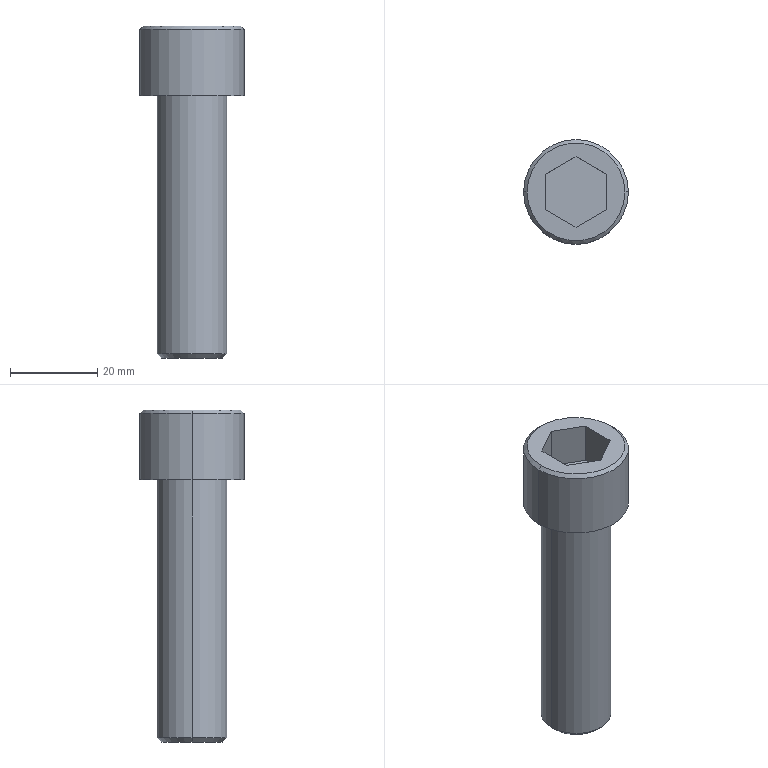Part | Creo | 1 solid | 18 faces | box 24 x 24 x 76 mm | volume 17625 mm3 | plane 10 | cylinder 4 | cone 4 | commonest cylinder face diameters 16 x2 24 x2
STEP:
#1=CARTESIAN_POINT('',(174.,251.,132.5));
#2=VERTEX_POINT('',#1);
#3=CARTESIAN_POINT('',(150.,251.,132.5));
#4=VERTEX_POINT('',#3);
#5=CARTESIAN_POINT('',(162.,251.,132.5));
#6=DIRECTION('',(0.,0.,-1.));
#7=DIRECTION('',(1.,0.,0.));
#8=AXIS2_PLACEMENT_3D('',#5,#6,#7);
#9=CIRCLE('',#8,12.);
#10=EDGE_CURVE('',#2,#4,#9,.T.);
#11=ORIENTED_EDGE('',*,*,#10,.F.);
#12=CARTESIAN_POINT('',(162.,251.,132.5));
#13=DIRECTION('',(0.,0.,-1.));
#14=DIRECTION('',(-1.,0.,0.));
#15=AXIS2_PLACEMENT_3D('',#12,#13,#14);
#16=CIRCLE('',#15,12.);
#17=EDGE_CURVE('',#4,#2,#16,.T.);
#18=ORIENTED_EDGE('',*,*,#17,.F.);
#19=EDGE_LOOP('',(#11,#18));
#20=FACE_OUTER_BOUND('',#19,.F.);
#21=CARTESIAN_POINT('',(154.,251.,132.5));
#22=VERTEX_POINT('',#21);
#23=CARTESIAN_POINT('',(170.,251.,132.5));
#24=VERTEX_POINT('',#23);
#25=CARTESIAN_POINT('',(162.,251.,132.5));
#26=DIRECTION('',(0.,0.,1.));
#27=DIRECTION('',(-1.,0.,0.));
#28=AXIS2_PLACEMENT_3D('',#25,#26,#27);
#29=CIRCLE('',#28,8.);
#30=EDGE_CURVE('',#22,#24,#29,.T.);
#31=ORIENTED_EDGE('',*,*,#30,.F.);
#32=CARTESIAN_POINT('',(162.,251.,132.5));
#33=DIRECTION('',(0.,0.,1.));
#34=DIRECTION('',(1.,0.,0.));
#35=AXIS2_PLACEMENT_3D('',#32,#33,#34);
#36=CIRCLE('',#35,8.);
#37=EDGE_CURVE('',#24,#22,#36,.T.);
#38=ORIENTED_EDGE('',*,*,#37,.F.);
#39=EDGE_LOOP('',(#31,#38));
#40=FACE_BOUND('',#39,.F.);
#41=CARTESIAN_POINT('',(162.,251.,132.5));
#42=DIRECTION('',(0.,0.,-1.));
#43=DIRECTION('',(-1.,0.,0.));
#44=AXIS2_PLACEMENT_3D('',#41,#42,#43);
#45=PLANE('',#44);
#46=ADVANCED_FACE('',(#20,#40),#45,.T.);
#47=CARTESIAN_POINT('',(170.,251.,73.5));
#48=VERTEX_POINT('',#47);
#49=CARTESIAN_POINT('',(154.,251.,73.5));
#50=VERTEX_POINT('',#49);
#51=CARTESIAN_POINT('',(162.,251.,73.5));
#52=DIRECTION('',(0.,0.,-1.));
#53=DIRECTION('',(1.,0.,0.));
#54=AXIS2_PLACEMENT_3D('',#51,#52,#53);
#55=CIRCLE('',#54,8.);
#56=EDGE_CURVE('',#48,#50,#55,.T.);
#57=ORIENTED_EDGE('',*,*,#56,.T.);
#58=CARTESIAN_POINT('',(154.,251.,132.5));
#59=DIRECTION('',(0.,0.,-1.));
#60=VECTOR('',#59,59.);
#61=LINE('',#58,#60);
#62=EDGE_CURVE('',#22,#50,#61,.T.);
#63=ORIENTED_EDGE('',*,*,#62,.F.);
#64=ORIENTED_EDGE('',*,*,#30,.T.);
#65=CARTESIAN_POINT('',(170.,251.,132.5));
#66=DIRECTION('',(0.,0.,-1.));
#67=VECTOR('',#66,59.);
#68=LINE('',#65,#67);
#69=EDGE_CURVE('',#24,#48,#68,.T.);
#70=ORIENTED_EDGE('',*,*,#69,.T.);
#71=EDGE_LOOP('',(#57,#63,#64,#70));
#72=FACE_OUTER_BOUND('',#71,.F.);
#73=CARTESIAN_POINT('',(162.,251.,150.5));
#74=DIRECTION('',(0.,0.,-1.));
#75=DIRECTION('',(-1.,0.,0.));
#76=AXIS2_PLACEMENT_3D('',#73,#74,#75);
#77=CYLINDRICAL_SURFACE('',#76,8.);
#78=ADVANCED_FACE('',(#72),#77,.T.);
#79=CARTESIAN_POINT('',(169.,251.,72.5));
#80=VERTEX_POINT('',#79);
#81=CARTESIAN_POINT('',(155.,251.,72.5));
#82=VERTEX_POINT('',#81);
#83=CARTESIAN_POINT('',(162.,251.,72.5));
#84=DIRECTION('',(0.,0.,-1.));
#85=DIRECTION('',(1.,0.,0.));
#86=AXIS2_PLACEMENT_3D('',#83,#84,#85);
#87=CIRCLE('',#86,7.);
#88=EDGE_CURVE('',#80,#82,#87,.T.);
#89=ORIENTED_EDGE('',*,*,#88,.T.);
#90=CARTESIAN_POINT('',(155.,251.,72.5));
#91=DIRECTION('',(-0.7071,0.,0.7071));
#92=VECTOR('',#91,1.414);
#93=LINE('',#90,#92);
#94=EDGE_CURVE('',#82,#50,#93,.T.);
#95=ORIENTED_EDGE('',*,*,#94,.T.);
#96=ORIENTED_EDGE('',*,*,#56,.F.);
#97=CARTESIAN_POINT('',(169.,251.,72.5));
#98=DIRECTION('',(0.7071,0.,0.7071));
#99=VECTOR('',#98,1.414);
#100=LINE('',#97,#99);
#101=EDGE_CURVE('',#80,#48,#100,.T.);
#102=ORIENTED_EDGE('',*,*,#101,.F.);
#103=EDGE_LOOP('',(#89,#95,#96,#102));
#104=FACE_OUTER_BOUND('',#103,.F.);
#105=CARTESIAN_POINT('',(162.,251.,73.));
#106=DIRECTION('',(0.,0.,1.));
#107=DIRECTION('',(1.,0.,0.));
#108=AXIS2_PLACEMENT_3D('',#105,#106,#107);
#109=CONICAL_SURFACE('',#108,7.5,45.);
#110=ADVANCED_FACE('',(#104),#109,.T.);
#111=CARTESIAN_POINT('',(162.,251.,72.5));
#112=DIRECTION('',(0.,0.,-1.));
#113=DIRECTION('',(-1.,0.,0.));
#114=AXIS2_PLACEMENT_3D('',#111,#112,#113);
#115=CIRCLE('',#114,7.);
#116=EDGE_CURVE('',#82,#80,#115,.T.);
#117=ORIENTED_EDGE('',*,*,#116,.F.);
#118=ORIENTED_EDGE('',*,*,#88,.F.);
#119=EDGE_LOOP('',(#117,#118));
#120=FACE_OUTER_BOUND('',#119,.F.);
#121=CARTESIAN_POINT('',(162.,251.,72.5));
#122=DIRECTION('',(0.,0.,-1.));
#123=DIRECTION('',(-1.,0.,0.));
#124=AXIS2_PLACEMENT_3D('',#121,#122,#123);
#125=PLANE('',#124);
#126=ADVANCED_FACE('',(#120),#125,.T.);
#127=ORIENTED_EDGE('',*,*,#116,.T.);
#128=ORIENTED_EDGE('',*,*,#101,.T.);
#129=CARTESIAN_POINT('',(162.,251.,73.5));
#130=DIRECTION('',(0.,0.,-1.));
#131=DIRECTION('',(-1.,0.,0.));
#132=AXIS2_PLACEMENT_3D('',#129,#130,#131);
#133=CIRCLE('',#132,8.);
#134=EDGE_CURVE('',#50,#48,#133,.T.);
#135=ORIENTED_EDGE('',*,*,#134,.F.);
#136=ORIENTED_EDGE('',*,*,#94,.F.);
#137=EDGE_LOOP('',(#127,#128,#135,#136));
#138=FACE_OUTER_BOUND('',#137,.F.);
#139=CARTESIAN_POINT('',(162.,251.,73.));
#140=DIRECTION('',(0.,0.,1.));
#141=DIRECTION('',(1.,0.,0.));
#142=AXIS2_PLACEMENT_3D('',#139,#140,#141);
#143=CONICAL_SURFACE('',#142,7.5,45.);
#144=ADVANCED_FACE('',(#138),#143,.T.);
#145=ORIENTED_EDGE('',*,*,#134,.T.);
#146=ORIENTED_EDGE('',*,*,#69,.F.);
#147=ORIENTED_EDGE('',*,*,#37,.T.);
#148=ORIENTED_EDGE('',*,*,#62,.T.);
#149=EDGE_LOOP('',(#145,#146,#147,#148));
#150=FACE_OUTER_BOUND('',#149,.F.);
#151=CARTESIAN_POINT('',(162.,251.,150.5));
#152=DIRECTION('',(0.,0.,-1.));
#153=DIRECTION('',(-1.,0.,0.));
#154=AXIS2_PLACEMENT_3D('',#151,#152,#153);
#155=CYLINDRICAL_SURFACE('',#154,8.);
#156=ADVANCED_FACE('',(#150),#155,.T.);
#157=CARTESIAN_POINT('',(150.,251.,147.7));
#158=VERTEX_POINT('',#157);
#159=CARTESIAN_POINT('',(174.,251.,147.7));
#160=VERTEX_POINT('',#159);
#161=CARTESIAN_POINT('',(162.,251.,147.7));
#162=DIRECTION('',(0.,0.,1.));
#163=DIRECTION('',(-1.,0.,0.));
#164=AXIS2_PLACEMENT_3D('',#161,#162,#163);
#165=CIRCLE('',#164,12.);
#166=EDGE_CURVE('',#158,#160,#165,.T.);
#167=ORIENTED_EDGE('',*,*,#166,.T.);
#168=CARTESIAN_POINT('',(174.,251.,147.7));
#169=DIRECTION('',(0.,0.,-1.));
#170=VECTOR('',#169,15.2);
#171=LINE('',#168,#170);
#172=EDGE_CURVE('',#160,#2,#171,.T.);
#173=ORIENTED_EDGE('',*,*,#172,.T.);
#174=ORIENTED_EDGE('',*,*,#10,.T.);
#175=CARTESIAN_POINT('',(150.,251.,147.7));
#176=DIRECTION('',(0.,0.,-1.));
#177=VECTOR('',#176,15.2);
#178=LINE('',#175,#177);
#179=EDGE_CURVE('',#158,#4,#178,.T.);
#180=ORIENTED_EDGE('',*,*,#179,.F.);
#181=EDGE_LOOP('',(#167,#173,#174,#180));
#182=FACE_OUTER_BOUND('',#181,.F.);
#183=CARTESIAN_POINT('',(162.,251.,150.5));
#184=DIRECTION('',(0.,0.,-1.));
#185=DIRECTION('',(-1.,0.,0.));
#186=AXIS2_PLACEMENT_3D('',#183,#184,#185);
#187=CYLINDRICAL_SURFACE('',#186,12.);
#188=ADVANCED_FACE('',(#182),#187,.T.);
#189=CARTESIAN_POINT('',(150.8,251.,148.5));
#190=VERTEX_POINT('',#189);
#191=CARTESIAN_POINT('',(173.2,251.,148.5));
#192=VERTEX_POINT('',#191);
#193=CARTESIAN_POINT('',(162.,251.,148.5));
#194=DIRECTION('',(0.,0.,1.));
#195=DIRECTION('',(-1.,0.,0.));
#196=AXIS2_PLACEMENT_3D('',#193,#194,#195);
#197=CIRCLE('',#196,11.2);
#198=EDGE_CURVE('',#190,#192,#197,.T.);
#199=ORIENTED_EDGE('',*,*,#198,.T.);
#200=CARTESIAN_POINT('',(173.2,251.,148.5));
#201=DIRECTION('',(0.7071,0.,-0.7071));
#202=VECTOR('',#201,1.131);
#203=LINE('',#200,#202);
#204=EDGE_CURVE('',#192,#160,#203,.T.);
#205=ORIENTED_EDGE('',*,*,#204,.T.);
#206=ORIENTED_EDGE('',*,*,#166,.F.);
#207=CARTESIAN_POINT('',(150.8,251.,148.5));
#208=DIRECTION('',(-0.7071,0.,-0.7071));
#209=VECTOR('',#208,1.131);
#210=LINE('',#207,#209);
#211=EDGE_CURVE('',#190,#158,#210,.T.);
#212=ORIENTED_EDGE('',*,*,#211,.F.);
#213=EDGE_LOOP('',(#199,#205,#206,#212));
#214=FACE_OUTER_BOUND('',#213,.F.);
#215=CARTESIAN_POINT('',(162.,251.,148.1));
#216=DIRECTION('',(0.,0.,-1.));
#217=DIRECTION('',(-1.,0.,0.));
#218=AXIS2_PLACEMENT_3D('',#215,#216,#217);
#219=CONICAL_SURFACE('',#218,11.6,45.);
#220=ADVANCED_FACE('',(#214),#219,.T.);
#221=ORIENTED_EDGE('',*,*,#198,.F.);
#222=CARTESIAN_POINT('',(162.,251.,148.5));
#223=DIRECTION('',(0.,0.,1.));
#224=DIRECTION('',(1.,0.,0.));
#225=AXIS2_PLACEMENT_3D('',#222,#223,#224);
#226=CIRCLE('',#225,11.2);
#227=EDGE_CURVE('',#192,#190,#226,.T.);
#228=ORIENTED_EDGE('',*,*,#227,.F.);
#229=EDGE_LOOP('',(#221,#228));
#230=FACE_OUTER_BOUND('',#229,.F.);
#231=CARTESIAN_POINT('',(169.,246.959,148.5));
#232=VERTEX_POINT('',#231);
#233=CARTESIAN_POINT('',(162.,242.917,148.5));
#234=VERTEX_POINT('',#233);
#235=CARTESIAN_POINT('',(169.,246.959,148.5));
#236=DIRECTION('',(-0.866,-0.5,0.));
#237=VECTOR('',#236,8.083);
#238=LINE('',#235,#237);
#239=EDGE_CURVE('',#232,#234,#238,.T.);
#240=ORIENTED_EDGE('',*,*,#239,.F.);
#241=CARTESIAN_POINT('',(169.,255.041,148.5));
#242=VERTEX_POINT('',#241);
#243=CARTESIAN_POINT('',(169.,255.041,148.5));
#244=DIRECTION('',(0.,-1.,0.));
#245=VECTOR('',#244,8.083);
#246=LINE('',#243,#245);
#247=EDGE_CURVE('',#242,#232,#246,.T.);
#248=ORIENTED_EDGE('',*,*,#247,.F.);
#249=CARTESIAN_POINT('',(162.,259.083,148.5));
#250=VERTEX_POINT('',#249);
#251=CARTESIAN_POINT('',(162.,259.083,148.5));
#252=DIRECTION('',(0.866,-0.5,0.));
#253=VECTOR('',#252,8.083);
#254=LINE('',#251,#253);
#255=EDGE_CURVE('',#250,#242,#254,.T.);
#256=ORIENTED_EDGE('',*,*,#255,.F.);
#257=CARTESIAN_POINT('',(155.,255.041,148.5));
#258=VERTEX_POINT('',#257);
#259=CARTESIAN_POINT('',(155.,255.041,148.5));
#260=DIRECTION('',(0.866,0.5,0.));
#261=VECTOR('',#260,8.083);
#262=LINE('',#259,#261);
#263=EDGE_CURVE('',#258,#250,#262,.T.);
#264=ORIENTED_EDGE('',*,*,#263,.F.);
#265=CARTESIAN_POINT('',(155.,246.959,148.5));
#266=VERTEX_POINT('',#265);
#267=CARTESIAN_POINT('',(155.,246.959,148.5));
#268=DIRECTION('',(0.,1.,0.));
#269=VECTOR('',#268,8.083);
#270=LINE('',#267,#269);
#271=EDGE_CURVE('',#266,#258,#270,.T.);
#272=ORIENTED_EDGE('',*,*,#271,.F.);
#273=CARTESIAN_POINT('',(162.,242.917,148.5));
#274=DIRECTION('',(-0.866,0.5,0.));
#275=VECTOR('',#274,8.083);
#276=LINE('',#273,#275);
#277=EDGE_CURVE('',#234,#266,#276,.T.);
#278=ORIENTED_EDGE('',*,*,#277,.F.);
#279=EDGE_LOOP('',(#240,#248,#256,#264,#272,#278));
#280=FACE_BOUND('',#279,.F.);
#281=CARTESIAN_POINT('',(162.,251.,148.5));
#282=DIRECTION('',(0.,0.,-1.));
#283=DIRECTION('',(-1.,0.,0.));
#284=AXIS2_PLACEMENT_3D('',#281,#282,#283);
#285=PLANE('',#284);
#286=ADVANCED_FACE('',(#230,#280),#285,.F.);
#287=ORIENTED_EDGE('',*,*,#227,.T.);
#288=ORIENTED_EDGE('',*,*,#211,.T.);
#289=CARTESIAN_POINT('',(162.,251.,147.7));
#290=DIRECTION('',(0.,0.,1.));
#291=DIRECTION('',(1.,0.,0.));
#292=AXIS2_PLACEMENT_3D('',#289,#290,#291);
#293=CIRCLE('',#292,12.);
#294=EDGE_CURVE('',#160,#158,#293,.T.);
#295=ORIENTED_EDGE('',*,*,#294,.F.);
#296=ORIENTED_EDGE('',*,*,#204,.F.);
#297=EDGE_LOOP('',(#287,#288,#295,#296));
#298=FACE_OUTER_BOUND('',#297,.F.);
#299=CARTESIAN_POINT('',(162.,251.,148.1));
#300=DIRECTION('',(0.,0.,-1.));
#301=DIRECTION('',(-1.,0.,0.));
#302=AXIS2_PLACEMENT_3D('',#299,#300,#301);
#303=CONICAL_SURFACE('',#302,11.6,45.);
#304=ADVANCED_FACE('',(#298),#303,.T.);
#305=ORIENTED_EDGE('',*,*,#294,.T.);
#306=ORIENTED_EDGE('',*,*,#179,.T.);
#307=ORIENTED_EDGE('',*,*,#17,.T.);
#308=ORIENTED_EDGE('',*,*,#172,.F.);
#309=EDGE_LOOP('',(#305,#306,#307,#308));
#310=FACE_OUTER_BOUND('',#309,.F.);
#311=CARTESIAN_POINT('',(162.,251.,150.5));
#312=DIRECTION('',(0.,0.,-1.));
#313=DIRECTION('',(-1.,0.,0.));
#314=AXIS2_PLACEMENT_3D('',#311,#312,#313);
#315=CYLINDRICAL_SURFACE('',#314,12.);
#316=ADVANCED_FACE('',(#310),#315,.T.);
#317=ORIENTED_EDGE('',*,*,#239,.T.);
#318=CARTESIAN_POINT('',(162.,242.917,138.9));
#319=VERTEX_POINT('',#318);
#320=CARTESIAN_POINT('',(162.,242.917,148.5));
#321=DIRECTION('',(0.,0.,-1.));
#322=VECTOR('',#321,9.6);
#323=LINE('',#320,#322);
#324=EDGE_CURVE('',#234,#319,#323,.T.);
#325=ORIENTED_EDGE('',*,*,#324,.T.);
#326=CARTESIAN_POINT('',(169.,246.959,138.9));
#327=VERTEX_POINT('',#326);
#328=CARTESIAN_POINT('',(162.,242.917,138.9));
#329=DIRECTION('',(0.866,0.5,0.));
#330=VECTOR('',#329,8.083);
#331=LINE('',#328,#330);
#332=EDGE_CURVE('',#319,#327,#331,.T.);
#333=ORIENTED_EDGE('',*,*,#332,.T.);
#334=CARTESIAN_POINT('',(169.,246.959,148.5));
#335=DIRECTION('',(0.,0.,-1.));
#336=VECTOR('',#335,9.6);
#337=LINE('',#334,#336);
#338=EDGE_CURVE('',#232,#327,#337,.T.);
#339=ORIENTED_EDGE('',*,*,#338,.F.);
#340=EDGE_LOOP('',(#317,#325,#333,#339));
#341=FACE_OUTER_BOUND('',#340,.F.);
#342=CARTESIAN_POINT('',(162.,242.917,138.9));
#343=DIRECTION('',(0.5,-0.866,0.));
#344=DIRECTION('',(0.866,0.5,0.));
#345=AXIS2_PLACEMENT_3D('',#342,#343,#344);
#346=PLANE('',#345);
#347=ADVANCED_FACE('',(#341),#346,.F.);
#348=ORIENTED_EDGE('',*,*,#277,.T.);
#349=CARTESIAN_POINT('',(155.,246.959,138.9));
#350=VERTEX_POINT('',#349);
#351=CARTESIAN_POINT('',(155.,246.959,148.5));
#352=DIRECTION('',(0.,0.,-1.));
#353=VECTOR('',#352,9.6);
#354=LINE('',#351,#353);
#355=EDGE_CURVE('',#266,#350,#354,.T.);
#356=ORIENTED_EDGE('',*,*,#355,.T.);
#357=CARTESIAN_POINT('',(155.,246.959,138.9));
#358=DIRECTION('',(0.866,-0.5,0.));
#359=VECTOR('',#358,8.083);
#360=LINE('',#357,#359);
#361=EDGE_CURVE('',#350,#319,#360,.T.);
#362=ORIENTED_EDGE('',*,*,#361,.T.);
#363=ORIENTED_EDGE('',*,*,#324,.F.);
#364=EDGE_LOOP('',(#348,#356,#362,#363));
#365=FACE_OUTER_BOUND('',#364,.F.);
#366=CARTESIAN_POINT('',(155.,246.959,138.9));
#367=DIRECTION('',(-0.5,-0.866,0.));
#368=DIRECTION('',(0.866,-0.5,0.));
#369=AXIS2_PLACEMENT_3D('',#366,#367,#368);
#370=PLANE('',#369);
#371=ADVANCED_FACE('',(#365),#370,.F.);
#372=ORIENTED_EDGE('',*,*,#271,.T.);
#373=CARTESIAN_POINT('',(155.,255.041,138.9));
#374=VERTEX_POINT('',#373);
#375=CARTESIAN_POINT('',(155.,255.041,148.5));
#376=DIRECTION('',(0.,0.,-1.));
#377=VECTOR('',#376,9.6);
#378=LINE('',#375,#377);
#379=EDGE_CURVE('',#258,#374,#378,.T.);
#380=ORIENTED_EDGE('',*,*,#379,.T.);
#381=CARTESIAN_POINT('',(155.,246.959,138.9));
#382=DIRECTION('',(0.,1.,0.));
#383=VECTOR('',#382,8.083);
#384=LINE('',#381,#383);
#385=EDGE_CURVE('',#350,#374,#384,.T.);
#386=ORIENTED_EDGE('',*,*,#385,.F.);
#387=ORIENTED_EDGE('',*,*,#355,.F.);
#388=EDGE_LOOP('',(#372,#380,#386,#387));
#389=FACE_OUTER_BOUND('',#388,.F.);
#390=CARTESIAN_POINT('',(155.,255.041,138.9));
#391=DIRECTION('',(-1.,0.,0.));
#392=DIRECTION('',(0.,0.,1.));
#393=AXIS2_PLACEMENT_3D('',#390,#391,#392);
#394=PLANE('',#393);
#395=ADVANCED_FACE('',(#389),#394,.F.);
#396=ORIENTED_EDGE('',*,*,#263,.T.);
#397=CARTESIAN_POINT('',(162.,259.083,138.9));
#398=VERTEX_POINT('',#397);
#399=CARTESIAN_POINT('',(162.,259.083,148.5));
#400=DIRECTION('',(0.,0.,-1.));
#401=VECTOR('',#400,9.6);
#402=LINE('',#399,#401);
#403=EDGE_CURVE('',#250,#398,#402,.T.);
#404=ORIENTED_EDGE('',*,*,#403,.T.);
#405=CARTESIAN_POINT('',(162.,259.083,138.9));
#406=DIRECTION('',(-0.866,-0.5,0.));
#407=VECTOR('',#406,8.083);
#408=LINE('',#405,#407);
#409=EDGE_CURVE('',#398,#374,#408,.T.);
#410=ORIENTED_EDGE('',*,*,#409,.T.);
#411=ORIENTED_EDGE('',*,*,#379,.F.);
#412=EDGE_LOOP('',(#396,#404,#410,#411));
#413=FACE_OUTER_BOUND('',#412,.F.);
#414=CARTESIAN_POINT('',(162.,259.083,138.9));
#415=DIRECTION('',(-0.5,0.866,0.));
#416=DIRECTION('',(-0.866,-0.5,0.));
#417=AXIS2_PLACEMENT_3D('',#414,#415,#416);
#418=PLANE('',#417);
#419=ADVANCED_FACE('',(#413),#418,.F.);
#420=ORIENTED_EDGE('',*,*,#255,.T.);
#421=CARTESIAN_POINT('',(169.,255.041,138.9));
#422=VERTEX_POINT('',#421);
#423=CARTESIAN_POINT('',(169.,255.041,148.5));
#424=DIRECTION('',(0.,0.,-1.));
#425=VECTOR('',#424,9.6);
#426=LINE('',#423,#425);
#427=EDGE_CURVE('',#242,#422,#426,.T.);
#428=ORIENTED_EDGE('',*,*,#427,.T.);
#429=CARTESIAN_POINT('',(169.,255.041,138.9));
#430=DIRECTION('',(-0.866,0.5,0.));
#431=VECTOR('',#430,8.083);
#432=LINE('',#429,#431);
#433=EDGE_CURVE('',#422,#398,#432,.T.);
#434=ORIENTED_EDGE('',*,*,#433,.T.);
#435=ORIENTED_EDGE('',*,*,#403,.F.);
#436=EDGE_LOOP('',(#420,#428,#434,#435));
#437=FACE_OUTER_BOUND('',#436,.F.);
#438=CARTESIAN_POINT('',(169.,255.041,138.9));
#439=DIRECTION('',(0.5,0.866,0.));
#440=DIRECTION('',(-0.866,0.5,0.));
#441=AXIS2_PLACEMENT_3D('',#438,#439,#440);
#442=PLANE('',#441);
#443=ADVANCED_FACE('',(#437),#442,.F.);
#444=ORIENTED_EDGE('',*,*,#247,.T.);
#445=ORIENTED_EDGE('',*,*,#338,.T.);
#446=CARTESIAN_POINT('',(169.,255.041,138.9));
#447=DIRECTION('',(0.,-1.,0.));
#448=VECTOR('',#447,8.083);
#449=LINE('',#446,#448);
#450=EDGE_CURVE('',#422,#327,#449,.T.);
#451=ORIENTED_EDGE('',*,*,#450,.F.);
#452=ORIENTED_EDGE('',*,*,#427,.F.);
#453=EDGE_LOOP('',(#444,#445,#451,#452));
#454=FACE_OUTER_BOUND('',#453,.F.);
#455=CARTESIAN_POINT('',(169.,246.959,138.9));
#456=DIRECTION('',(1.,0.,0.));
#457=DIRECTION('',(0.,0.,-1.));
#458=AXIS2_PLACEMENT_3D('',#455,#456,#457);
#459=PLANE('',#458);
#460=ADVANCED_FACE('',(#454),#459,.F.);
#461=ORIENTED_EDGE('',*,*,#361,.F.);
#462=ORIENTED_EDGE('',*,*,#385,.T.);
#463=ORIENTED_EDGE('',*,*,#409,.F.);
#464=ORIENTED_EDGE('',*,*,#433,.F.);
#465=ORIENTED_EDGE('',*,*,#450,.T.);
#466=ORIENTED_EDGE('',*,*,#332,.F.);
#467=EDGE_LOOP('',(#461,#462,#463,#464,#465,#466));
#468=FACE_OUTER_BOUND('',#467,.F.);
#469=CARTESIAN_POINT('',(148.,251.,138.9));
#470=DIRECTION('',(0.,0.,-1.));
#471=DIRECTION('',(-1.,0.,0.));
#472=AXIS2_PLACEMENT_3D('',#469,#470,#471);
#473=PLANE('',#472);
#474=ADVANCED_FACE('',(#468),#473,.F.);
#475=CLOSED_SHELL('',(#46,#78,#110,#126,#144,#156,#188,#220,#286,#304,#316,#347,#371,#395,#419,#443,#460,#474));
#476=MANIFOLD_SOLID_BREP('',#475);
#477=(LENGTH_UNIT()NAMED_UNIT(*)SI_UNIT(.MILLI.,.METRE.));
#478=UNCERTAINTY_MEASURE_WITH_UNIT(LENGTH_MEASURE(0.008324),#477,'','');
#479=(NAMED_UNIT(*)PLANE_ANGLE_UNIT()SI_UNIT($,.RADIAN.));
#480=PLANE_ANGLE_MEASURE_WITH_UNIT(PLANE_ANGLE_MEASURE(0.01745),#479);
#481=(CONVERSION_BASED_UNIT('DEGREE',#480)NAMED_UNIT(*)PLANE_ANGLE_UNIT());
#482=(NAMED_UNIT(*)SI_UNIT($,.STERADIAN.)SOLID_ANGLE_UNIT());
#483=(GEOMETRIC_REPRESENTATION_CONTEXT(3)GLOBAL_UNCERTAINTY_ASSIGNED_CONTEXT((#478))GLOBAL_UNIT_ASSIGNED_CONTEXT((#477,#481,#482))REPRESENTATION_CONTEXT('',''));
#484=ADVANCED_BREP_SHAPE_REPRESENTATION('',(#476),#483);